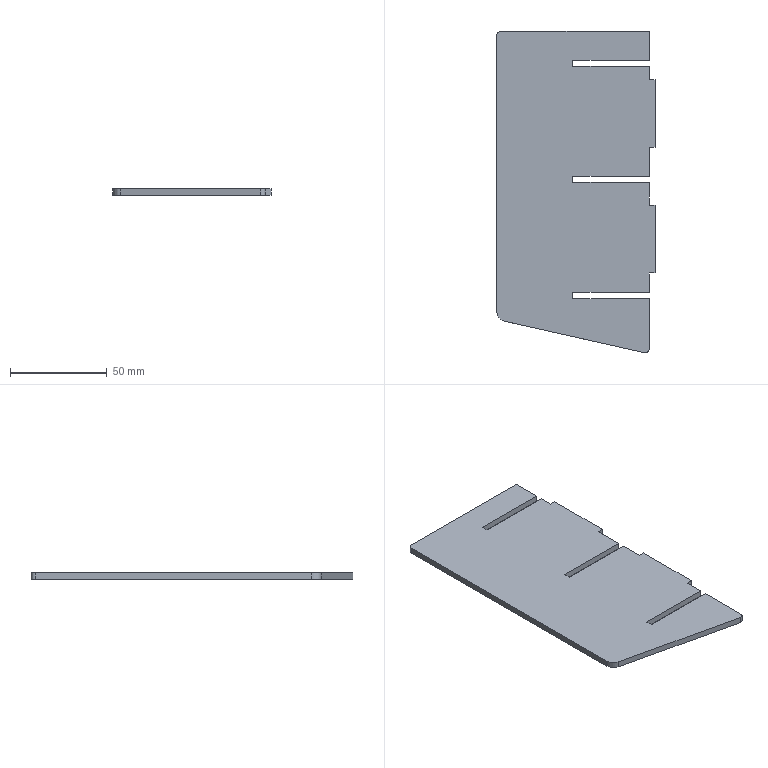Part | SolidWorks | features FlatPattern 1, SMBaseFlange 1, SheetMetal 1 | 1 solid | 29 faces | box 81.8 x 166.27 x 3.2 mm | volume 39259 mm3 | plane 26 | cylinder 3 | commonest cylinder face diameters 4 x2 10 x1
STEP:
#1=CARTESIAN_POINT('',(-280.,-76.17,0.));
#2=VERTEX_POINT('',#1);
#3=CARTESIAN_POINT('',(-276.098,-81.048,0.));
#4=VERTEX_POINT('',#3);
#5=CARTESIAN_POINT('',(-275.,-76.17,0.));
#6=DIRECTION('',(0.,0.,1.));
#7=DIRECTION('',(1.,0.,0.));
#8=AXIS2_PLACEMENT_3D('',#5,#6,#7);
#9=CIRCLE('',#8,5.);
#10=EDGE_CURVE('',#2,#4,#9,.T.);
#11=ORIENTED_EDGE('',*,*,#10,.T.);
#12=CARTESIAN_POINT('',(-276.098,-81.048,3.2));
#13=VERTEX_POINT('',#12);
#14=CARTESIAN_POINT('',(-276.098,-81.048,3.2));
#15=DIRECTION('',(0.,0.,-1.));
#16=VECTOR('',#15,1000.);
#17=LINE('',#14,#16);
#18=EDGE_CURVE('',#13,#4,#17,.T.);
#19=ORIENTED_EDGE('',*,*,#18,.F.);
#20=CARTESIAN_POINT('',(-280.,-76.17,3.2));
#21=VERTEX_POINT('',#20);
#22=CARTESIAN_POINT('',(-275.,-76.17,3.2));
#23=DIRECTION('',(0.,0.,1.));
#24=DIRECTION('',(1.,0.,0.));
#25=AXIS2_PLACEMENT_3D('',#22,#23,#24);
#26=CIRCLE('',#25,5.);
#27=EDGE_CURVE('',#21,#13,#26,.T.);
#28=ORIENTED_EDGE('',*,*,#27,.F.);
#29=CARTESIAN_POINT('',(-280.,-76.17,3.2));
#30=DIRECTION('',(0.,0.,-1.));
#31=VECTOR('',#30,1000.);
#32=LINE('',#29,#31);
#33=EDGE_CURVE('',#21,#2,#32,.T.);
#34=ORIENTED_EDGE('',*,*,#33,.T.);
#35=EDGE_LOOP('',(#11,#19,#28,#34));
#36=FACE_OUTER_BOUND('',#35,.T.);
#37=CARTESIAN_POINT('',(-275.,-76.17,3.2));
#38=DIRECTION('',(0.,0.,-1.));
#39=DIRECTION('',(-1.,0.,0.));
#40=AXIS2_PLACEMENT_3D('',#37,#38,#39);
#41=CYLINDRICAL_SURFACE('',#40,5.);
#42=ADVANCED_FACE('',(#36),#41,.T.);
#43=CARTESIAN_POINT('',(-203.639,-97.351,0.));
#44=VERTEX_POINT('',#43);
#45=CARTESIAN_POINT('',(-276.098,-81.048,0.));
#46=DIRECTION('',(0.9756,-0.2195,0.));
#47=VECTOR('',#46,1000.);
#48=LINE('',#45,#47);
#49=EDGE_CURVE('',#4,#44,#48,.T.);
#50=ORIENTED_EDGE('',*,*,#49,.T.);
#51=CARTESIAN_POINT('',(-203.639,-97.351,3.2));
#52=VERTEX_POINT('',#51);
#53=CARTESIAN_POINT('',(-203.639,-97.351,3.2));
#54=DIRECTION('',(0.,0.,-1.));
#55=VECTOR('',#54,1000.);
#56=LINE('',#53,#55);
#57=EDGE_CURVE('',#52,#44,#56,.T.);
#58=ORIENTED_EDGE('',*,*,#57,.F.);
#59=CARTESIAN_POINT('',(-276.098,-81.048,3.2));
#60=DIRECTION('',(0.9756,-0.2195,0.));
#61=VECTOR('',#60,1000.);
#62=LINE('',#59,#61);
#63=EDGE_CURVE('',#13,#52,#62,.T.);
#64=ORIENTED_EDGE('',*,*,#63,.F.);
#65=ORIENTED_EDGE('',*,*,#18,.T.);
#66=EDGE_LOOP('',(#50,#58,#64,#65));
#67=FACE_OUTER_BOUND('',#66,.T.);
#68=CARTESIAN_POINT('',(-276.098,-81.048,3.2));
#69=DIRECTION('',(0.2195,0.9756,0.));
#70=DIRECTION('',(-0.9756,0.2195,0.));
#71=AXIS2_PLACEMENT_3D('',#68,#69,#70);
#72=PLANE('',#71);
#73=ADVANCED_FACE('',(#67),#72,.F.);
#74=CARTESIAN_POINT('',(-201.2,-95.4,0.));
#75=VERTEX_POINT('',#74);
#76=CARTESIAN_POINT('',(-203.2,-95.4,0.));
#77=DIRECTION('',(0.,0.,1.));
#78=DIRECTION('',(-1.,0.,0.));
#79=AXIS2_PLACEMENT_3D('',#76,#77,#78);
#80=CIRCLE('',#79,2.);
#81=EDGE_CURVE('',#44,#75,#80,.T.);
#82=ORIENTED_EDGE('',*,*,#81,.T.);
#83=CARTESIAN_POINT('',(-201.2,-95.4,3.2));
#84=VERTEX_POINT('',#83);
#85=CARTESIAN_POINT('',(-201.2,-95.4,3.2));
#86=DIRECTION('',(0.,0.,-1.));
#87=VECTOR('',#86,1000.);
#88=LINE('',#85,#87);
#89=EDGE_CURVE('',#84,#75,#88,.T.);
#90=ORIENTED_EDGE('',*,*,#89,.F.);
#91=CARTESIAN_POINT('',(-203.2,-95.4,3.2));
#92=DIRECTION('',(0.,0.,1.));
#93=DIRECTION('',(-1.,0.,0.));
#94=AXIS2_PLACEMENT_3D('',#91,#92,#93);
#95=CIRCLE('',#94,2.);
#96=EDGE_CURVE('',#52,#84,#95,.T.);
#97=ORIENTED_EDGE('',*,*,#96,.F.);
#98=ORIENTED_EDGE('',*,*,#57,.T.);
#99=EDGE_LOOP('',(#82,#90,#97,#98));
#100=FACE_OUTER_BOUND('',#99,.T.);
#101=CARTESIAN_POINT('',(-203.2,-95.4,3.2));
#102=DIRECTION('',(0.,0.,-1.));
#103=DIRECTION('',(-1.,0.,0.));
#104=AXIS2_PLACEMENT_3D('',#101,#102,#103);
#105=CYLINDRICAL_SURFACE('',#104,2.);
#106=ADVANCED_FACE('',(#100),#105,.T.);
#107=CARTESIAN_POINT('',(-201.2,-69.33,0.));
#108=VERTEX_POINT('',#107);
#109=CARTESIAN_POINT('',(-201.2,-95.4,0.));
#110=DIRECTION('',(0.,1.,0.));
#111=VECTOR('',#110,1000.);
#112=LINE('',#109,#111);
#113=EDGE_CURVE('',#75,#108,#112,.T.);
#114=ORIENTED_EDGE('',*,*,#113,.T.);
#115=CARTESIAN_POINT('',(-201.2,-69.33,3.2));
#116=VERTEX_POINT('',#115);
#117=CARTESIAN_POINT('',(-201.2,-69.33,3.2));
#118=DIRECTION('',(0.,0.,-1.));
#119=VECTOR('',#118,1000.);
#120=LINE('',#117,#119);
#121=EDGE_CURVE('',#116,#108,#120,.T.);
#122=ORIENTED_EDGE('',*,*,#121,.F.);
#123=CARTESIAN_POINT('',(-201.2,-95.4,3.2));
#124=DIRECTION('',(0.,1.,0.));
#125=VECTOR('',#124,1000.);
#126=LINE('',#123,#125);
#127=EDGE_CURVE('',#84,#116,#126,.T.);
#128=ORIENTED_EDGE('',*,*,#127,.F.);
#129=ORIENTED_EDGE('',*,*,#89,.T.);
#130=EDGE_LOOP('',(#114,#122,#128,#129));
#131=FACE_OUTER_BOUND('',#130,.T.);
#132=CARTESIAN_POINT('',(-201.2,-95.4,3.2));
#133=DIRECTION('',(-1.,0.,0.));
#134=DIRECTION('',(0.,-1.,0.));
#135=AXIS2_PLACEMENT_3D('',#132,#133,#134);
#136=PLANE('',#135);
#137=ADVANCED_FACE('',(#131),#136,.F.);
#138=CARTESIAN_POINT('',(-240.7,-69.33,0.));
#139=VERTEX_POINT('',#138);
#140=CARTESIAN_POINT('',(-240.7,-69.33,0.));
#141=DIRECTION('',(-1.,0.,0.));
#142=VECTOR('',#141,1000.);
#143=LINE('',#140,#142);
#144=EDGE_CURVE('',#108,#139,#143,.T.);
#145=ORIENTED_EDGE('',*,*,#144,.T.);
#146=CARTESIAN_POINT('',(-240.7,-69.33,3.2));
#147=VERTEX_POINT('',#146);
#148=CARTESIAN_POINT('',(-240.7,-69.33,3.2));
#149=DIRECTION('',(0.,0.,-1.));
#150=VECTOR('',#149,1000.);
#151=LINE('',#148,#150);
#152=EDGE_CURVE('',#147,#139,#151,.T.);
#153=ORIENTED_EDGE('',*,*,#152,.F.);
#154=CARTESIAN_POINT('',(-240.7,-69.33,3.2));
#155=DIRECTION('',(-1.,0.,0.));
#156=VECTOR('',#155,1000.);
#157=LINE('',#154,#156);
#158=EDGE_CURVE('',#116,#147,#157,.T.);
#159=ORIENTED_EDGE('',*,*,#158,.F.);
#160=ORIENTED_EDGE('',*,*,#121,.T.);
#161=EDGE_LOOP('',(#145,#153,#159,#160));
#162=FACE_OUTER_BOUND('',#161,.T.);
#163=CARTESIAN_POINT('',(-240.7,-69.33,3.2));
#164=DIRECTION('',(0.,-1.,0.));
#165=DIRECTION('',(0.,0.,-1.));
#166=AXIS2_PLACEMENT_3D('',#163,#164,#165);
#167=PLANE('',#166);
#168=ADVANCED_FACE('',(#162),#167,.F.);
#169=CARTESIAN_POINT('',(-240.7,-66.13,0.));
#170=VERTEX_POINT('',#169);
#171=CARTESIAN_POINT('',(-240.7,-66.13,0.));
#172=DIRECTION('',(0.,1.,0.));
#173=VECTOR('',#172,1000.);
#174=LINE('',#171,#173);
#175=EDGE_CURVE('',#139,#170,#174,.T.);
#176=ORIENTED_EDGE('',*,*,#175,.T.);
#177=CARTESIAN_POINT('',(-240.7,-66.13,3.2));
#178=VERTEX_POINT('',#177);
#179=CARTESIAN_POINT('',(-240.7,-66.13,3.2));
#180=DIRECTION('',(0.,0.,-1.));
#181=VECTOR('',#180,1000.);
#182=LINE('',#179,#181);
#183=EDGE_CURVE('',#178,#170,#182,.T.);
#184=ORIENTED_EDGE('',*,*,#183,.F.);
#185=CARTESIAN_POINT('',(-240.7,-66.13,3.2));
#186=DIRECTION('',(0.,1.,0.));
#187=VECTOR('',#186,1000.);
#188=LINE('',#185,#187);
#189=EDGE_CURVE('',#147,#178,#188,.T.);
#190=ORIENTED_EDGE('',*,*,#189,.F.);
#191=ORIENTED_EDGE('',*,*,#152,.T.);
#192=EDGE_LOOP('',(#176,#184,#190,#191));
#193=FACE_OUTER_BOUND('',#192,.T.);
#194=CARTESIAN_POINT('',(-240.7,-66.13,3.2));
#195=DIRECTION('',(-1.,0.,0.));
#196=DIRECTION('',(0.,0.,1.));
#197=AXIS2_PLACEMENT_3D('',#194,#195,#196);
#198=PLANE('',#197);
#199=ADVANCED_FACE('',(#193),#198,.F.);
#200=CARTESIAN_POINT('',(-201.2,-66.13,0.));
#201=VERTEX_POINT('',#200);
#202=CARTESIAN_POINT('',(-201.2,-66.13,0.));
#203=DIRECTION('',(1.,0.,0.));
#204=VECTOR('',#203,1000.);
#205=LINE('',#202,#204);
#206=EDGE_CURVE('',#170,#201,#205,.T.);
#207=ORIENTED_EDGE('',*,*,#206,.T.);
#208=CARTESIAN_POINT('',(-201.2,-66.13,3.2));
#209=VERTEX_POINT('',#208);
#210=CARTESIAN_POINT('',(-201.2,-66.13,3.2));
#211=DIRECTION('',(0.,0.,-1.));
#212=VECTOR('',#211,1000.);
#213=LINE('',#210,#212);
#214=EDGE_CURVE('',#209,#201,#213,.T.);
#215=ORIENTED_EDGE('',*,*,#214,.F.);
#216=CARTESIAN_POINT('',(-201.2,-66.13,3.2));
#217=DIRECTION('',(1.,0.,0.));
#218=VECTOR('',#217,1000.);
#219=LINE('',#216,#218);
#220=EDGE_CURVE('',#178,#209,#219,.T.);
#221=ORIENTED_EDGE('',*,*,#220,.F.);
#222=ORIENTED_EDGE('',*,*,#183,.T.);
#223=EDGE_LOOP('',(#207,#215,#221,#222));
#224=FACE_OUTER_BOUND('',#223,.T.);
#225=CARTESIAN_POINT('',(-201.2,-66.13,3.2));
#226=DIRECTION('',(0.,1.,0.));
#227=DIRECTION('',(0.,0.,1.));
#228=AXIS2_PLACEMENT_3D('',#225,#226,#227);
#229=PLANE('',#228);
#230=ADVANCED_FACE('',(#224),#229,.F.);
#231=CARTESIAN_POINT('',(-201.2,-56.13,0.));
#232=VERTEX_POINT('',#231);
#233=CARTESIAN_POINT('',(-201.2,-66.13,0.));
#234=DIRECTION('',(0.,1.,0.));
#235=VECTOR('',#234,1000.);
#236=LINE('',#233,#235);
#237=EDGE_CURVE('',#201,#232,#236,.T.);
#238=ORIENTED_EDGE('',*,*,#237,.T.);
#239=CARTESIAN_POINT('',(-201.2,-56.13,3.2));
#240=VERTEX_POINT('',#239);
#241=CARTESIAN_POINT('',(-201.2,-56.13,3.2));
#242=DIRECTION('',(0.,0.,-1.));
#243=VECTOR('',#242,1000.);
#244=LINE('',#241,#243);
#245=EDGE_CURVE('',#240,#232,#244,.T.);
#246=ORIENTED_EDGE('',*,*,#245,.F.);
#247=CARTESIAN_POINT('',(-201.2,-66.13,3.2));
#248=DIRECTION('',(0.,1.,0.));
#249=VECTOR('',#248,1000.);
#250=LINE('',#247,#249);
#251=EDGE_CURVE('',#209,#240,#250,.T.);
#252=ORIENTED_EDGE('',*,*,#251,.F.);
#253=ORIENTED_EDGE('',*,*,#214,.T.);
#254=EDGE_LOOP('',(#238,#246,#252,#253));
#255=FACE_OUTER_BOUND('',#254,.T.);
#256=CARTESIAN_POINT('',(-201.2,-66.13,3.2));
#257=DIRECTION('',(-1.,0.,0.));
#258=DIRECTION('',(0.,-1.,0.));
#259=AXIS2_PLACEMENT_3D('',#256,#257,#258);
#260=PLANE('',#259);
#261=ADVANCED_FACE('',(#255),#260,.F.);
#262=CARTESIAN_POINT('',(-198.2,-56.13,0.));
#263=VERTEX_POINT('',#262);
#264=CARTESIAN_POINT('',(-201.2,-56.13,0.));
#265=DIRECTION('',(1.,0.,0.));
#266=VECTOR('',#265,1000.);
#267=LINE('',#264,#266);
#268=EDGE_CURVE('',#232,#263,#267,.T.);
#269=ORIENTED_EDGE('',*,*,#268,.T.);
#270=CARTESIAN_POINT('',(-198.2,-56.13,3.2));
#271=VERTEX_POINT('',#270);
#272=CARTESIAN_POINT('',(-198.2,-56.13,3.2));
#273=DIRECTION('',(0.,0.,-1.));
#274=VECTOR('',#273,1000.);
#275=LINE('',#272,#274);
#276=EDGE_CURVE('',#271,#263,#275,.T.);
#277=ORIENTED_EDGE('',*,*,#276,.F.);
#278=CARTESIAN_POINT('',(-201.2,-56.13,3.2));
#279=DIRECTION('',(1.,0.,0.));
#280=VECTOR('',#279,1000.);
#281=LINE('',#278,#280);
#282=EDGE_CURVE('',#240,#271,#281,.T.);
#283=ORIENTED_EDGE('',*,*,#282,.F.);
#284=ORIENTED_EDGE('',*,*,#245,.T.);
#285=EDGE_LOOP('',(#269,#277,#283,#284));
#286=FACE_OUTER_BOUND('',#285,.T.);
#287=CARTESIAN_POINT('',(-201.2,-56.13,3.2));
#288=DIRECTION('',(0.,1.,0.));
#289=DIRECTION('',(0.,0.,1.));
#290=AXIS2_PLACEMENT_3D('',#287,#288,#289);
#291=PLANE('',#290);
#292=ADVANCED_FACE('',(#286),#291,.F.);
#293=CARTESIAN_POINT('',(-198.2,-21.13,0.));
#294=VERTEX_POINT('',#293);
#295=CARTESIAN_POINT('',(-198.2,-56.13,0.));
#296=DIRECTION('',(0.,1.,0.));
#297=VECTOR('',#296,1000.);
#298=LINE('',#295,#297);
#299=EDGE_CURVE('',#263,#294,#298,.T.);
#300=ORIENTED_EDGE('',*,*,#299,.T.);
#301=CARTESIAN_POINT('',(-198.2,-21.13,3.2));
#302=VERTEX_POINT('',#301);
#303=CARTESIAN_POINT('',(-198.2,-21.13,3.2));
#304=DIRECTION('',(0.,0.,-1.));
#305=VECTOR('',#304,1000.);
#306=LINE('',#303,#305);
#307=EDGE_CURVE('',#302,#294,#306,.T.);
#308=ORIENTED_EDGE('',*,*,#307,.F.);
#309=CARTESIAN_POINT('',(-198.2,-56.13,3.2));
#310=DIRECTION('',(0.,1.,0.));
#311=VECTOR('',#310,1000.);
#312=LINE('',#309,#311);
#313=EDGE_CURVE('',#271,#302,#312,.T.);
#314=ORIENTED_EDGE('',*,*,#313,.F.);
#315=ORIENTED_EDGE('',*,*,#276,.T.);
#316=EDGE_LOOP('',(#300,#308,#314,#315));
#317=FACE_OUTER_BOUND('',#316,.T.);
#318=CARTESIAN_POINT('',(-198.2,-56.13,3.2));
#319=DIRECTION('',(-1.,0.,0.));
#320=DIRECTION('',(0.,0.,1.));
#321=AXIS2_PLACEMENT_3D('',#318,#319,#320);
#322=PLANE('',#321);
#323=ADVANCED_FACE('',(#317),#322,.F.);
#324=CARTESIAN_POINT('',(-201.2,-21.13,0.));
#325=VERTEX_POINT('',#324);
#326=CARTESIAN_POINT('',(-198.2,-21.13,0.));
#327=DIRECTION('',(-1.,0.,0.));
#328=VECTOR('',#327,1000.);
#329=LINE('',#326,#328);
#330=EDGE_CURVE('',#294,#325,#329,.T.);
#331=ORIENTED_EDGE('',*,*,#330,.T.);
#332=CARTESIAN_POINT('',(-201.2,-21.13,3.2));
#333=VERTEX_POINT('',#332);
#334=CARTESIAN_POINT('',(-201.2,-21.13,3.2));
#335=DIRECTION('',(0.,0.,-1.));
#336=VECTOR('',#335,1000.);
#337=LINE('',#334,#336);
#338=EDGE_CURVE('',#333,#325,#337,.T.);
#339=ORIENTED_EDGE('',*,*,#338,.F.);
#340=CARTESIAN_POINT('',(-198.2,-21.13,3.2));
#341=DIRECTION('',(-1.,0.,0.));
#342=VECTOR('',#341,1000.);
#343=LINE('',#340,#342);
#344=EDGE_CURVE('',#302,#333,#343,.T.);
#345=ORIENTED_EDGE('',*,*,#344,.F.);
#346=ORIENTED_EDGE('',*,*,#307,.T.);
#347=EDGE_LOOP('',(#331,#339,#345,#346));
#348=FACE_OUTER_BOUND('',#347,.T.);
#349=CARTESIAN_POINT('',(-198.2,-21.13,3.2));
#350=DIRECTION('',(0.,-1.,0.));
#351=DIRECTION('',(0.,0.,-1.));
#352=AXIS2_PLACEMENT_3D('',#349,#350,#351);
#353=PLANE('',#352);
#354=ADVANCED_FACE('',(#348),#353,.F.);
#355=CARTESIAN_POINT('',(-201.2,-9.33,0.));
#356=VERTEX_POINT('',#355);
#357=CARTESIAN_POINT('',(-201.2,-21.13,0.));
#358=DIRECTION('',(0.,1.,0.));
#359=VECTOR('',#358,1000.);
#360=LINE('',#357,#359);
#361=EDGE_CURVE('',#325,#356,#360,.T.);
#362=ORIENTED_EDGE('',*,*,#361,.T.);
#363=CARTESIAN_POINT('',(-201.2,-9.33,3.2));
#364=VERTEX_POINT('',#363);
#365=CARTESIAN_POINT('',(-201.2,-9.33,3.2));
#366=DIRECTION('',(0.,0.,-1.));
#367=VECTOR('',#366,1000.);
#368=LINE('',#365,#367);
#369=EDGE_CURVE('',#364,#356,#368,.T.);
#370=ORIENTED_EDGE('',*,*,#369,.F.);
#371=CARTESIAN_POINT('',(-201.2,-21.13,3.2));
#372=DIRECTION('',(0.,1.,0.));
#373=VECTOR('',#372,1000.);
#374=LINE('',#371,#373);
#375=EDGE_CURVE('',#333,#364,#374,.T.);
#376=ORIENTED_EDGE('',*,*,#375,.F.);
#377=ORIENTED_EDGE('',*,*,#338,.T.);
#378=EDGE_LOOP('',(#362,#370,#376,#377));
#379=FACE_OUTER_BOUND('',#378,.T.);
#380=CARTESIAN_POINT('',(-201.2,-21.13,3.2));
#381=DIRECTION('',(-1.,0.,0.));
#382=DIRECTION('',(0.,-1.,0.));
#383=AXIS2_PLACEMENT_3D('',#380,#381,#382);
#384=PLANE('',#383);
#385=ADVANCED_FACE('',(#379),#384,.F.);
#386=CARTESIAN_POINT('',(-240.7,-9.33,0.));
#387=VERTEX_POINT('',#386);
#388=CARTESIAN_POINT('',(-240.7,-9.33,0.));
#389=DIRECTION('',(-1.,0.,0.));
#390=VECTOR('',#389,1000.);
#391=LINE('',#388,#390);
#392=EDGE_CURVE('',#356,#387,#391,.T.);
#393=ORIENTED_EDGE('',*,*,#392,.T.);
#394=CARTESIAN_POINT('',(-240.7,-9.33,3.2));
#395=VERTEX_POINT('',#394);
#396=CARTESIAN_POINT('',(-240.7,-9.33,3.2));
#397=DIRECTION('',(0.,0.,-1.));
#398=VECTOR('',#397,1000.);
#399=LINE('',#396,#398);
#400=EDGE_CURVE('',#395,#387,#399,.T.);
#401=ORIENTED_EDGE('',*,*,#400,.F.);
#402=CARTESIAN_POINT('',(-240.7,-9.33,3.2));
#403=DIRECTION('',(-1.,0.,0.));
#404=VECTOR('',#403,1000.);
#405=LINE('',#402,#404);
#406=EDGE_CURVE('',#364,#395,#405,.T.);
#407=ORIENTED_EDGE('',*,*,#406,.F.);
#408=ORIENTED_EDGE('',*,*,#369,.T.);
#409=EDGE_LOOP('',(#393,#401,#407,#408));
#410=FACE_OUTER_BOUND('',#409,.T.);
#411=CARTESIAN_POINT('',(-240.7,-9.33,3.2));
#412=DIRECTION('',(0.,-1.,0.));
#413=DIRECTION('',(0.,0.,-1.));
#414=AXIS2_PLACEMENT_3D('',#411,#412,#413);
#415=PLANE('',#414);
#416=ADVANCED_FACE('',(#410),#415,.F.);
#417=CARTESIAN_POINT('',(-240.7,-6.13,0.));
#418=VERTEX_POINT('',#417);
#419=CARTESIAN_POINT('',(-240.7,-6.13,0.));
#420=DIRECTION('',(0.,1.,0.));
#421=VECTOR('',#420,1000.);
#422=LINE('',#419,#421);
#423=EDGE_CURVE('',#387,#418,#422,.T.);
#424=ORIENTED_EDGE('',*,*,#423,.T.);
#425=CARTESIAN_POINT('',(-240.7,-6.13,3.2));
#426=VERTEX_POINT('',#425);
#427=CARTESIAN_POINT('',(-240.7,-6.13,3.2));
#428=DIRECTION('',(0.,0.,-1.));
#429=VECTOR('',#428,1000.);
#430=LINE('',#427,#429);
#431=EDGE_CURVE('',#426,#418,#430,.T.);
#432=ORIENTED_EDGE('',*,*,#431,.F.);
#433=CARTESIAN_POINT('',(-240.7,-6.13,3.2));
#434=DIRECTION('',(0.,1.,0.));
#435=VECTOR('',#434,1000.);
#436=LINE('',#433,#435);
#437=EDGE_CURVE('',#395,#426,#436,.T.);
#438=ORIENTED_EDGE('',*,*,#437,.F.);
#439=ORIENTED_EDGE('',*,*,#400,.T.);
#440=EDGE_LOOP('',(#424,#432,#438,#439));
#441=FACE_OUTER_BOUND('',#440,.T.);
#442=CARTESIAN_POINT('',(-240.7,-6.13,3.2));
#443=DIRECTION('',(-1.,0.,0.));
#444=DIRECTION('',(0.,0.,1.));
#445=AXIS2_PLACEMENT_3D('',#442,#443,#444);
#446=PLANE('',#445);
#447=ADVANCED_FACE('',(#441),#446,.F.);
#448=CARTESIAN_POINT('',(-201.2,-6.13,0.));
#449=VERTEX_POINT('',#448);
#450=CARTESIAN_POINT('',(-201.2,-6.13,0.));
#451=DIRECTION('',(1.,0.,0.));
#452=VECTOR('',#451,1000.);
#453=LINE('',#450,#452);
#454=EDGE_CURVE('',#418,#449,#453,.T.);
#455=ORIENTED_EDGE('',*,*,#454,.T.);
#456=CARTESIAN_POINT('',(-201.2,-6.13,3.2));
#457=VERTEX_POINT('',#456);
#458=CARTESIAN_POINT('',(-201.2,-6.13,3.2));
#459=DIRECTION('',(0.,0.,-1.));
#460=VECTOR('',#459,1000.);
#461=LINE('',#458,#460);
#462=EDGE_CURVE('',#457,#449,#461,.T.);
#463=ORIENTED_EDGE('',*,*,#462,.F.);
#464=CARTESIAN_POINT('',(-201.2,-6.13,3.2));
#465=DIRECTION('',(1.,0.,0.));
#466=VECTOR('',#465,1000.);
#467=LINE('',#464,#466);
#468=EDGE_CURVE('',#426,#457,#467,.T.);
#469=ORIENTED_EDGE('',*,*,#468,.F.);
#470=ORIENTED_EDGE('',*,*,#431,.T.);
#471=EDGE_LOOP('',(#455,#463,#469,#470));
#472=FACE_OUTER_BOUND('',#471,.T.);
#473=CARTESIAN_POINT('',(-201.2,-6.13,3.2));
#474=DIRECTION('',(0.,1.,0.));
#475=DIRECTION('',(-1.,0.,0.));
#476=AXIS2_PLACEMENT_3D('',#473,#474,#475);
#477=PLANE('',#476);
#478=ADVANCED_FACE('',(#472),#477,.F.);
#479=CARTESIAN_POINT('',(-201.2,8.87,0.));
#480=VERTEX_POINT('',#479);
#481=CARTESIAN_POINT('',(-201.2,-6.13,0.));
#482=DIRECTION('',(0.,1.,0.));
#483=VECTOR('',#482,1000.);
#484=LINE('',#481,#483);
#485=EDGE_CURVE('',#449,#480,#484,.T.);
#486=ORIENTED_EDGE('',*,*,#485,.T.);
#487=CARTESIAN_POINT('',(-201.2,8.87,3.2));
#488=VERTEX_POINT('',#487);
#489=CARTESIAN_POINT('',(-201.2,8.87,3.2));
#490=DIRECTION('',(0.,0.,-1.));
#491=VECTOR('',#490,1000.);
#492=LINE('',#489,#491);
#493=EDGE_CURVE('',#488,#480,#492,.T.);
#494=ORIENTED_EDGE('',*,*,#493,.F.);
#495=CARTESIAN_POINT('',(-201.2,-6.13,3.2));
#496=DIRECTION('',(0.,1.,0.));
#497=VECTOR('',#496,1000.);
#498=LINE('',#495,#497);
#499=EDGE_CURVE('',#457,#488,#498,.T.);
#500=ORIENTED_EDGE('',*,*,#499,.F.);
#501=ORIENTED_EDGE('',*,*,#462,.T.);
#502=EDGE_LOOP('',(#486,#494,#500,#501));
#503=FACE_OUTER_BOUND('',#502,.T.);
#504=CARTESIAN_POINT('',(-201.2,-6.13,3.2));
#505=DIRECTION('',(-1.,0.,0.));
#506=DIRECTION('',(0.,-1.,0.));
#507=AXIS2_PLACEMENT_3D('',#504,#505,#506);
#508=PLANE('',#507);
#509=ADVANCED_FACE('',(#503),#508,.F.);
#510=CARTESIAN_POINT('',(-198.2,8.87,0.));
#511=VERTEX_POINT('',#510);
#512=CARTESIAN_POINT('',(-201.2,8.87,0.));
#513=DIRECTION('',(1.,0.,0.));
#514=VECTOR('',#513,1000.);
#515=LINE('',#512,#514);
#516=EDGE_CURVE('',#480,#511,#515,.T.);
#517=ORIENTED_EDGE('',*,*,#516,.T.);
#518=CARTESIAN_POINT('',(-198.2,8.87,3.2));
#519=VERTEX_POINT('',#518);
#520=CARTESIAN_POINT('',(-198.2,8.87,3.2));
#521=DIRECTION('',(0.,0.,-1.));
#522=VECTOR('',#521,1000.);
#523=LINE('',#520,#522);
#524=EDGE_CURVE('',#519,#511,#523,.T.);
#525=ORIENTED_EDGE('',*,*,#524,.F.);
#526=CARTESIAN_POINT('',(-201.2,8.87,3.2));
#527=DIRECTION('',(1.,0.,0.));
#528=VECTOR('',#527,1000.);
#529=LINE('',#526,#528);
#530=EDGE_CURVE('',#488,#519,#529,.T.);
#531=ORIENTED_EDGE('',*,*,#530,.F.);
#532=ORIENTED_EDGE('',*,*,#493,.T.);
#533=EDGE_LOOP('',(#517,#525,#531,#532));
#534=FACE_OUTER_BOUND('',#533,.T.);
#535=CARTESIAN_POINT('',(-201.2,8.87,3.2));
#536=DIRECTION('',(0.,1.,0.));
#537=DIRECTION('',(0.,0.,1.));
#538=AXIS2_PLACEMENT_3D('',#535,#536,#537);
#539=PLANE('',#538);
#540=ADVANCED_FACE('',(#534),#539,.F.);
#541=CARTESIAN_POINT('',(-198.2,43.87,0.));
#542=VERTEX_POINT('',#541);
#543=CARTESIAN_POINT('',(-198.2,8.87,0.));
#544=DIRECTION('',(0.,1.,0.));
#545=VECTOR('',#544,1000.);
#546=LINE('',#543,#545);
#547=EDGE_CURVE('',#511,#542,#546,.T.);
#548=ORIENTED_EDGE('',*,*,#547,.T.);
#549=CARTESIAN_POINT('',(-198.2,43.87,3.2));
#550=VERTEX_POINT('',#549);
#551=CARTESIAN_POINT('',(-198.2,43.87,3.2));
#552=DIRECTION('',(0.,0.,-1.));
#553=VECTOR('',#552,1000.);
#554=LINE('',#551,#553);
#555=EDGE_CURVE('',#550,#542,#554,.T.);
#556=ORIENTED_EDGE('',*,*,#555,.F.);
#557=CARTESIAN_POINT('',(-198.2,8.87,3.2));
#558=DIRECTION('',(0.,1.,0.));
#559=VECTOR('',#558,1000.);
#560=LINE('',#557,#559);
#561=EDGE_CURVE('',#519,#550,#560,.T.);
#562=ORIENTED_EDGE('',*,*,#561,.F.);
#563=ORIENTED_EDGE('',*,*,#524,.T.);
#564=EDGE_LOOP('',(#548,#556,#562,#563));
#565=FACE_OUTER_BOUND('',#564,.T.);
#566=CARTESIAN_POINT('',(-198.2,8.87,3.2));
#567=DIRECTION('',(-1.,0.,0.));
#568=DIRECTION('',(0.,0.,1.));
#569=AXIS2_PLACEMENT_3D('',#566,#567,#568);
#570=PLANE('',#569);
#571=ADVANCED_FACE('',(#565),#570,.F.);
#572=CARTESIAN_POINT('',(-201.2,43.87,0.));
#573=VERTEX_POINT('',#572);
#574=CARTESIAN_POINT('',(-198.2,43.87,0.));
#575=DIRECTION('',(-1.,0.,0.));
#576=VECTOR('',#575,1000.);
#577=LINE('',#574,#576);
#578=EDGE_CURVE('',#542,#573,#577,.T.);
#579=ORIENTED_EDGE('',*,*,#578,.T.);
#580=CARTESIAN_POINT('',(-201.2,43.87,3.2));
#581=VERTEX_POINT('',#580);
#582=CARTESIAN_POINT('',(-201.2,43.87,3.2));
#583=DIRECTION('',(0.,0.,-1.));
#584=VECTOR('',#583,1000.);
#585=LINE('',#582,#584);
#586=EDGE_CURVE('',#581,#573,#585,.T.);
#587=ORIENTED_EDGE('',*,*,#586,.F.);
#588=CARTESIAN_POINT('',(-198.2,43.87,3.2));
#589=DIRECTION('',(-1.,0.,0.));
#590=VECTOR('',#589,1000.);
#591=LINE('',#588,#590);
#592=EDGE_CURVE('',#550,#581,#591,.T.);
#593=ORIENTED_EDGE('',*,*,#592,.F.);
#594=ORIENTED_EDGE('',*,*,#555,.T.);
#595=EDGE_LOOP('',(#579,#587,#593,#594));
#596=FACE_OUTER_BOUND('',#595,.T.);
#597=CARTESIAN_POINT('',(-198.2,43.87,3.2));
#598=DIRECTION('',(0.,-1.,0.));
#599=DIRECTION('',(0.,0.,-1.));
#600=AXIS2_PLACEMENT_3D('',#597,#598,#599);
#601=PLANE('',#600);
#602=ADVANCED_FACE('',(#596),#601,.F.);
#603=CARTESIAN_POINT('',(-201.2,50.67,0.));
#604=VERTEX_POINT('',#603);
#605=CARTESIAN_POINT('',(-201.2,43.87,0.));
#606=DIRECTION('',(0.,1.,0.));
#607=VECTOR('',#606,1000.);
#608=LINE('',#605,#607);
#609=EDGE_CURVE('',#573,#604,#608,.T.);
#610=ORIENTED_EDGE('',*,*,#609,.T.);
#611=CARTESIAN_POINT('',(-201.2,50.67,3.2));
#612=VERTEX_POINT('',#611);
#613=CARTESIAN_POINT('',(-201.2,50.67,3.2));
#614=DIRECTION('',(0.,0.,-1.));
#615=VECTOR('',#614,1000.);
#616=LINE('',#613,#615);
#617=EDGE_CURVE('',#612,#604,#616,.T.);
#618=ORIENTED_EDGE('',*,*,#617,.F.);
#619=CARTESIAN_POINT('',(-201.2,43.87,3.2));
#620=DIRECTION('',(0.,1.,0.));
#621=VECTOR('',#620,1000.);
#622=LINE('',#619,#621);
#623=EDGE_CURVE('',#581,#612,#622,.T.);
#624=ORIENTED_EDGE('',*,*,#623,.F.);
#625=ORIENTED_EDGE('',*,*,#586,.T.);
#626=EDGE_LOOP('',(#610,#618,#624,#625));
#627=FACE_OUTER_BOUND('',#626,.T.);
#628=CARTESIAN_POINT('',(-201.2,43.87,3.2));
#629=DIRECTION('',(-1.,0.,0.));
#630=DIRECTION('',(0.,-1.,0.));
#631=AXIS2_PLACEMENT_3D('',#628,#629,#630);
#632=PLANE('',#631);
#633=ADVANCED_FACE('',(#627),#632,.F.);
#634=CARTESIAN_POINT('',(-240.7,50.67,0.));
#635=VERTEX_POINT('',#634);
#636=CARTESIAN_POINT('',(-240.7,50.67,0.));
#637=DIRECTION('',(-1.,0.,0.));
#638=VECTOR('',#637,1000.);
#639=LINE('',#636,#638);
#640=EDGE_CURVE('',#604,#635,#639,.T.);
#641=ORIENTED_EDGE('',*,*,#640,.T.);
#642=CARTESIAN_POINT('',(-240.7,50.67,3.2));
#643=VERTEX_POINT('',#642);
#644=CARTESIAN_POINT('',(-240.7,50.67,3.2));
#645=DIRECTION('',(0.,0.,-1.));
#646=VECTOR('',#645,1000.);
#647=LINE('',#644,#646);
#648=EDGE_CURVE('',#643,#635,#647,.T.);
#649=ORIENTED_EDGE('',*,*,#648,.F.);
#650=CARTESIAN_POINT('',(-240.7,50.67,3.2));
#651=DIRECTION('',(-1.,0.,0.));
#652=VECTOR('',#651,1000.);
#653=LINE('',#650,#652);
#654=EDGE_CURVE('',#612,#643,#653,.T.);
#655=ORIENTED_EDGE('',*,*,#654,.F.);
#656=ORIENTED_EDGE('',*,*,#617,.T.);
#657=EDGE_LOOP('',(#641,#649,#655,#656));
#658=FACE_OUTER_BOUND('',#657,.T.);
#659=CARTESIAN_POINT('',(-240.7,50.67,3.2));
#660=DIRECTION('',(0.,-1.,0.));
#661=DIRECTION('',(0.,0.,-1.));
#662=AXIS2_PLACEMENT_3D('',#659,#660,#661);
#663=PLANE('',#662);
#664=ADVANCED_FACE('',(#658),#663,.F.);
#665=CARTESIAN_POINT('',(-240.7,53.87,0.));
#666=VERTEX_POINT('',#665);
#667=CARTESIAN_POINT('',(-240.7,53.87,0.));
#668=DIRECTION('',(0.,1.,0.));
#669=VECTOR('',#668,1000.);
#670=LINE('',#667,#669);
#671=EDGE_CURVE('',#635,#666,#670,.T.);
#672=ORIENTED_EDGE('',*,*,#671,.T.);
#673=CARTESIAN_POINT('',(-240.7,53.87,3.2));
#674=VERTEX_POINT('',#673);
#675=CARTESIAN_POINT('',(-240.7,53.87,3.2));
#676=DIRECTION('',(0.,0.,-1.));
#677=VECTOR('',#676,1000.);
#678=LINE('',#675,#677);
#679=EDGE_CURVE('',#674,#666,#678,.T.);
#680=ORIENTED_EDGE('',*,*,#679,.F.);
#681=CARTESIAN_POINT('',(-240.7,53.87,3.2));
#682=DIRECTION('',(0.,1.,0.));
#683=VECTOR('',#682,1000.);
#684=LINE('',#681,#683);
#685=EDGE_CURVE('',#643,#674,#684,.T.);
#686=ORIENTED_EDGE('',*,*,#685,.F.);
#687=ORIENTED_EDGE('',*,*,#648,.T.);
#688=EDGE_LOOP('',(#672,#680,#686,#687));
#689=FACE_OUTER_BOUND('',#688,.T.);
#690=CARTESIAN_POINT('',(-240.7,53.87,3.2));
#691=DIRECTION('',(-1.,0.,0.));
#692=DIRECTION('',(0.,0.,1.));
#693=AXIS2_PLACEMENT_3D('',#690,#691,#692);
#694=PLANE('',#693);
#695=ADVANCED_FACE('',(#689),#694,.F.);
#696=CARTESIAN_POINT('',(-201.2,53.87,0.));
#697=VERTEX_POINT('',#696);
#698=CARTESIAN_POINT('',(-201.2,53.87,0.));
#699=DIRECTION('',(1.,0.,0.));
#700=VECTOR('',#699,1000.);
#701=LINE('',#698,#700);
#702=EDGE_CURVE('',#666,#697,#701,.T.);
#703=ORIENTED_EDGE('',*,*,#702,.T.);
#704=CARTESIAN_POINT('',(-201.2,53.87,3.2));
#705=VERTEX_POINT('',#704);
#706=CARTESIAN_POINT('',(-201.2,53.87,3.2));
#707=DIRECTION('',(0.,0.,-1.));
#708=VECTOR('',#707,1000.);
#709=LINE('',#706,#708);
#710=EDGE_CURVE('',#705,#697,#709,.T.);
#711=ORIENTED_EDGE('',*,*,#710,.F.);
#712=CARTESIAN_POINT('',(-201.2,53.87,3.2));
#713=DIRECTION('',(1.,0.,0.));
#714=VECTOR('',#713,1000.);
#715=LINE('',#712,#714);
#716=EDGE_CURVE('',#674,#705,#715,.T.);
#717=ORIENTED_EDGE('',*,*,#716,.F.);
#718=ORIENTED_EDGE('',*,*,#679,.T.);
#719=EDGE_LOOP('',(#703,#711,#717,#718));
#720=FACE_OUTER_BOUND('',#719,.T.);
#721=CARTESIAN_POINT('',(-201.2,53.87,3.2));
#722=DIRECTION('',(0.,1.,0.));
#723=DIRECTION('',(-1.,0.,0.));
#724=AXIS2_PLACEMENT_3D('',#721,#722,#723);
#725=PLANE('',#724);
#726=ADVANCED_FACE('',(#720),#725,.F.);
#727=CARTESIAN_POINT('',(-201.2,68.87,0.));
#728=VERTEX_POINT('',#727);
#729=CARTESIAN_POINT('',(-201.2,53.87,0.));
#730=DIRECTION('',(0.,1.,0.));
#731=VECTOR('',#730,1000.);
#732=LINE('',#729,#731);
#733=EDGE_CURVE('',#697,#728,#732,.T.);
#734=ORIENTED_EDGE('',*,*,#733,.T.);
#735=CARTESIAN_POINT('',(-201.2,68.87,3.2));
#736=VERTEX_POINT('',#735);
#737=CARTESIAN_POINT('',(-201.2,68.87,3.2));
#738=DIRECTION('',(0.,0.,-1.));
#739=VECTOR('',#738,1000.);
#740=LINE('',#737,#739);
#741=EDGE_CURVE('',#736,#728,#740,.T.);
#742=ORIENTED_EDGE('',*,*,#741,.F.);
#743=CARTESIAN_POINT('',(-201.2,53.87,3.2));
#744=DIRECTION('',(0.,1.,0.));
#745=VECTOR('',#744,1000.);
#746=LINE('',#743,#745);
#747=EDGE_CURVE('',#705,#736,#746,.T.);
#748=ORIENTED_EDGE('',*,*,#747,.F.);
#749=ORIENTED_EDGE('',*,*,#710,.T.);
#750=EDGE_LOOP('',(#734,#742,#748,#749));
#751=FACE_OUTER_BOUND('',#750,.T.);
#752=CARTESIAN_POINT('',(-201.2,53.87,3.2));
#753=DIRECTION('',(-1.,0.,0.));
#754=DIRECTION('',(0.,-1.,0.));
#755=AXIS2_PLACEMENT_3D('',#752,#753,#754);
#756=PLANE('',#755);
#757=ADVANCED_FACE('',(#751),#756,.F.);
#758=CARTESIAN_POINT('',(-278.,68.87,0.));
#759=VERTEX_POINT('',#758);
#760=CARTESIAN_POINT('',(-201.2,68.87,0.));
#761=DIRECTION('',(-1.,0.,0.));
#762=VECTOR('',#761,1000.);
#763=LINE('',#760,#762);
#764=EDGE_CURVE('',#728,#759,#763,.T.);
#765=ORIENTED_EDGE('',*,*,#764,.T.);
#766=CARTESIAN_POINT('',(-278.,68.87,3.2));
#767=VERTEX_POINT('',#766);
#768=CARTESIAN_POINT('',(-278.,68.87,3.2));
#769=DIRECTION('',(0.,0.,-1.));
#770=VECTOR('',#769,1000.);
#771=LINE('',#768,#770);
#772=EDGE_CURVE('',#767,#759,#771,.T.);
#773=ORIENTED_EDGE('',*,*,#772,.F.);
#774=CARTESIAN_POINT('',(-201.2,68.87,3.2));
#775=DIRECTION('',(-1.,0.,0.));
#776=VECTOR('',#775,1000.);
#777=LINE('',#774,#776);
#778=EDGE_CURVE('',#736,#767,#777,.T.);
#779=ORIENTED_EDGE('',*,*,#778,.F.);
#780=ORIENTED_EDGE('',*,*,#741,.T.);
#781=EDGE_LOOP('',(#765,#773,#779,#780));
#782=FACE_OUTER_BOUND('',#781,.T.);
#783=CARTESIAN_POINT('',(-201.2,68.87,3.2));
#784=DIRECTION('',(0.,-1.,0.));
#785=DIRECTION('',(1.,0.,0.));
#786=AXIS2_PLACEMENT_3D('',#783,#784,#785);
#787=PLANE('',#786);
#788=ADVANCED_FACE('',(#782),#787,.F.);
#789=CARTESIAN_POINT('',(-280.,66.87,0.));
#790=VERTEX_POINT('',#789);
#791=CARTESIAN_POINT('',(-278.,66.87,0.));
#792=DIRECTION('',(0.,0.,1.));
#793=DIRECTION('',(-1.,0.,0.));
#794=AXIS2_PLACEMENT_3D('',#791,#792,#793);
#795=CIRCLE('',#794,2.);
#796=EDGE_CURVE('',#759,#790,#795,.T.);
#797=ORIENTED_EDGE('',*,*,#796,.T.);
#798=CARTESIAN_POINT('',(-280.,66.87,3.2));
#799=VERTEX_POINT('',#798);
#800=CARTESIAN_POINT('',(-280.,66.87,3.2));
#801=DIRECTION('',(0.,0.,-1.));
#802=VECTOR('',#801,1000.);
#803=LINE('',#800,#802);
#804=EDGE_CURVE('',#799,#790,#803,.T.);
#805=ORIENTED_EDGE('',*,*,#804,.F.);
#806=CARTESIAN_POINT('',(-278.,66.87,3.2));
#807=DIRECTION('',(0.,0.,1.));
#808=DIRECTION('',(-1.,0.,0.));
#809=AXIS2_PLACEMENT_3D('',#806,#807,#808);
#810=CIRCLE('',#809,2.);
#811=EDGE_CURVE('',#767,#799,#810,.T.);
#812=ORIENTED_EDGE('',*,*,#811,.F.);
#813=ORIENTED_EDGE('',*,*,#772,.T.);
#814=EDGE_LOOP('',(#797,#805,#812,#813));
#815=FACE_OUTER_BOUND('',#814,.T.);
#816=CARTESIAN_POINT('',(-278.,66.87,3.2));
#817=DIRECTION('',(0.,0.,-1.));
#818=DIRECTION('',(-1.,0.,0.));
#819=AXIS2_PLACEMENT_3D('',#816,#817,#818);
#820=CYLINDRICAL_SURFACE('',#819,2.);
#821=ADVANCED_FACE('',(#815),#820,.T.);
#822=CARTESIAN_POINT('',(-280.,66.87,0.));
#823=DIRECTION('',(0.,-1.,0.));
#824=VECTOR('',#823,1000.);
#825=LINE('',#822,#824);
#826=EDGE_CURVE('',#790,#2,#825,.T.);
#827=ORIENTED_EDGE('',*,*,#826,.T.);
#828=ORIENTED_EDGE('',*,*,#33,.F.);
#829=CARTESIAN_POINT('',(-280.,66.87,3.2));
#830=DIRECTION('',(0.,-1.,0.));
#831=VECTOR('',#830,1000.);
#832=LINE('',#829,#831);
#833=EDGE_CURVE('',#799,#21,#832,.T.);
#834=ORIENTED_EDGE('',*,*,#833,.F.);
#835=ORIENTED_EDGE('',*,*,#804,.T.);
#836=EDGE_LOOP('',(#827,#828,#834,#835));
#837=FACE_OUTER_BOUND('',#836,.T.);
#838=CARTESIAN_POINT('',(-280.,66.87,3.2));
#839=DIRECTION('',(1.,0.,0.));
#840=DIRECTION('',(0.,0.,-1.));
#841=AXIS2_PLACEMENT_3D('',#838,#839,#840);
#842=PLANE('',#841);
#843=ADVANCED_FACE('',(#837),#842,.F.);
#844=ORIENTED_EDGE('',*,*,#27,.T.);
#845=ORIENTED_EDGE('',*,*,#63,.T.);
#846=ORIENTED_EDGE('',*,*,#96,.T.);
#847=ORIENTED_EDGE('',*,*,#127,.T.);
#848=ORIENTED_EDGE('',*,*,#158,.T.);
#849=ORIENTED_EDGE('',*,*,#189,.T.);
#850=ORIENTED_EDGE('',*,*,#220,.T.);
#851=ORIENTED_EDGE('',*,*,#251,.T.);
#852=ORIENTED_EDGE('',*,*,#282,.T.);
#853=ORIENTED_EDGE('',*,*,#313,.T.);
#854=ORIENTED_EDGE('',*,*,#344,.T.);
#855=ORIENTED_EDGE('',*,*,#375,.T.);
#856=ORIENTED_EDGE('',*,*,#406,.T.);
#857=ORIENTED_EDGE('',*,*,#437,.T.);
#858=ORIENTED_EDGE('',*,*,#468,.T.);
#859=ORIENTED_EDGE('',*,*,#499,.T.);
#860=ORIENTED_EDGE('',*,*,#530,.T.);
#861=ORIENTED_EDGE('',*,*,#561,.T.);
#862=ORIENTED_EDGE('',*,*,#592,.T.);
#863=ORIENTED_EDGE('',*,*,#623,.T.);
#864=ORIENTED_EDGE('',*,*,#654,.T.);
#865=ORIENTED_EDGE('',*,*,#685,.T.);
#866=ORIENTED_EDGE('',*,*,#716,.T.);
#867=ORIENTED_EDGE('',*,*,#747,.T.);
#868=ORIENTED_EDGE('',*,*,#778,.T.);
#869=ORIENTED_EDGE('',*,*,#811,.T.);
#870=ORIENTED_EDGE('',*,*,#833,.T.);
#871=EDGE_LOOP('',(#844,#845,#846,#847,#848,#849,#850,#851,#852,#853,#854,#855,#856,#857,#858,#859,#860,#861,#862,#863,#864,#865,#866,#867,#868,#869,#870));
#872=FACE_OUTER_BOUND('',#871,.T.);
#873=CARTESIAN_POINT('',(-275.,-76.17,3.2));
#874=DIRECTION('',(0.,0.,1.));
#875=DIRECTION('',(1.,0.,0.));
#876=AXIS2_PLACEMENT_3D('',#873,#874,#875);
#877=PLANE('',#876);
#878=ADVANCED_FACE('',(#872),#877,.T.);
#879=ORIENTED_EDGE('',*,*,#10,.F.);
#880=ORIENTED_EDGE('',*,*,#826,.F.);
#881=ORIENTED_EDGE('',*,*,#796,.F.);
#882=ORIENTED_EDGE('',*,*,#764,.F.);
#883=ORIENTED_EDGE('',*,*,#733,.F.);
#884=ORIENTED_EDGE('',*,*,#702,.F.);
#885=ORIENTED_EDGE('',*,*,#671,.F.);
#886=ORIENTED_EDGE('',*,*,#640,.F.);
#887=ORIENTED_EDGE('',*,*,#609,.F.);
#888=ORIENTED_EDGE('',*,*,#578,.F.);
#889=ORIENTED_EDGE('',*,*,#547,.F.);
#890=ORIENTED_EDGE('',*,*,#516,.F.);
#891=ORIENTED_EDGE('',*,*,#485,.F.);
#892=ORIENTED_EDGE('',*,*,#454,.F.);
#893=ORIENTED_EDGE('',*,*,#423,.F.);
#894=ORIENTED_EDGE('',*,*,#392,.F.);
#895=ORIENTED_EDGE('',*,*,#361,.F.);
#896=ORIENTED_EDGE('',*,*,#330,.F.);
#897=ORIENTED_EDGE('',*,*,#299,.F.);
#898=ORIENTED_EDGE('',*,*,#268,.F.);
#899=ORIENTED_EDGE('',*,*,#237,.F.);
#900=ORIENTED_EDGE('',*,*,#206,.F.);
#901=ORIENTED_EDGE('',*,*,#175,.F.);
#902=ORIENTED_EDGE('',*,*,#144,.F.);
#903=ORIENTED_EDGE('',*,*,#113,.F.);
#904=ORIENTED_EDGE('',*,*,#81,.F.);
#905=ORIENTED_EDGE('',*,*,#49,.F.);
#906=EDGE_LOOP('',(#879,#880,#881,#882,#883,#884,#885,#886,#887,#888,#889,#890,#891,#892,#893,#894,#895,#896,#897,#898,#899,#900,#901,#902,#903,#904,#905));
#907=FACE_OUTER_BOUND('',#906,.T.);
#908=CARTESIAN_POINT('',(-275.,-76.17,0.));
#909=DIRECTION('',(0.,0.,1.));
#910=DIRECTION('',(1.,0.,0.));
#911=AXIS2_PLACEMENT_3D('',#908,#909,#910);
#912=PLANE('',#911);
#913=ADVANCED_FACE('',(#907),#912,.F.);
#914=CLOSED_SHELL('',(#42,#73,#106,#137,#168,#199,#230,#261,#292,#323,#354,#385,#416,#447,#478,#509,#540,#571,#602,#633,#664,#695,#726,#757,#788,#821,#843,#878,#913));
#915=MANIFOLD_SOLID_BREP('',#914);
#916=CARTESIAN_POINT('',(0.,0.,0.));
#917=DIRECTION('',(0.,0.,1.));
#918=DIRECTION('',(1.,0.,0.));
#919=AXIS2_PLACEMENT_3D('',#916,#917,#918);
#920=(LENGTH_UNIT()NAMED_UNIT(*)SI_UNIT(.MILLI.,.METRE.));
#921=UNCERTAINTY_MEASURE_WITH_UNIT(LENGTH_MEASURE(0.00001),#920,'','');
#922=(NAMED_UNIT(*)PLANE_ANGLE_UNIT()SI_UNIT($,.RADIAN.));
#923=(NAMED_UNIT(*)SI_UNIT($,.STERADIAN.)SOLID_ANGLE_UNIT());
#924=(GEOMETRIC_REPRESENTATION_CONTEXT(3)GLOBAL_UNCERTAINTY_ASSIGNED_CONTEXT((#921))GLOBAL_UNIT_ASSIGNED_CONTEXT((#920,#922,#923))REPRESENTATION_CONTEXT('',''));
#925=ADVANCED_BREP_SHAPE_REPRESENTATION('',(#915,#919),#924);